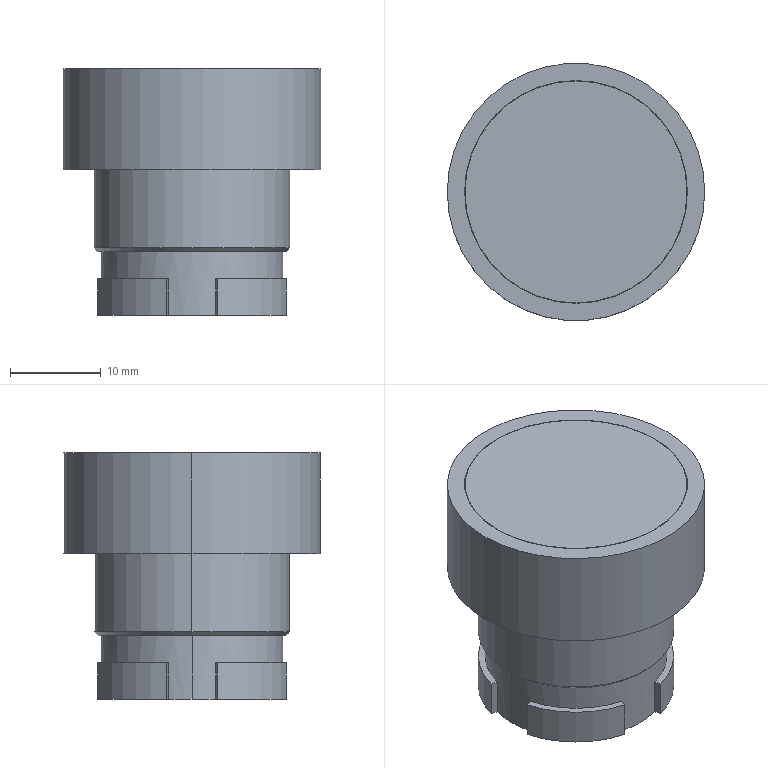Part | STEP file | 001. Yiweide green push-button switch EB6-BA31 | 1 solid | 40 faces | box 28.3 x 28.3 x 27.1 mm | volume 9249 mm3 | plane 20 | cylinder 18 | cone 2 | commonest cylinder face diameters 21.5 x6 18 x2 20 x2 24.4 x2 24.5 x2 26 x2
STEP:
#1=CARTESIAN_POINT('',(9.,0.,-4.));
#2=VERTEX_POINT('',#1);
#3=CARTESIAN_POINT('',(-9.,0.,-4.));
#4=VERTEX_POINT('',#3);
#5=CARTESIAN_POINT('',(0.,0.,-4.));
#6=DIRECTION('',(0.,0.,-1.));
#7=DIRECTION('',(-1.,0.,0.));
#8=AXIS2_PLACEMENT_3D('',#5,#6,#7);
#9=CIRCLE('',#8,9.);
#10=EDGE_CURVE('',#2,#4,#9,.T.);
#11=ORIENTED_EDGE('',*,*,#10,.F.);
#12=CARTESIAN_POINT('',(9.,0.,-16.));
#13=VERTEX_POINT('',#12);
#14=CARTESIAN_POINT('',(9.,0.,-4.));
#15=DIRECTION('',(0.,0.,-1.));
#16=VECTOR('',#15,1000.);
#17=LINE('',#14,#16);
#18=EDGE_CURVE('',#2,#13,#17,.T.);
#19=ORIENTED_EDGE('',*,*,#18,.T.);
#20=CARTESIAN_POINT('',(-9.,0.,-16.));
#21=VERTEX_POINT('',#20);
#22=CARTESIAN_POINT('',(0.,0.,-16.));
#23=DIRECTION('',(0.,0.,-1.));
#24=DIRECTION('',(-1.,0.,0.));
#25=AXIS2_PLACEMENT_3D('',#22,#23,#24);
#26=CIRCLE('',#25,9.);
#27=EDGE_CURVE('',#13,#21,#26,.T.);
#28=ORIENTED_EDGE('',*,*,#27,.T.);
#29=CARTESIAN_POINT('',(-9.,0.,-4.));
#30=DIRECTION('',(0.,0.,-1.));
#31=VECTOR('',#30,1000.);
#32=LINE('',#29,#31);
#33=EDGE_CURVE('',#4,#21,#32,.T.);
#34=ORIENTED_EDGE('',*,*,#33,.F.);
#35=EDGE_LOOP('',(#11,#19,#28,#34));
#36=FACE_OUTER_BOUND('',#35,.T.);
#37=CARTESIAN_POINT('',(0.,0.,-4.));
#38=DIRECTION('',(0.,0.,-1.));
#39=DIRECTION('',(-1.,0.,0.));
#40=AXIS2_PLACEMENT_3D('',#37,#38,#39);
#41=CYLINDRICAL_SURFACE('',#40,9.);
#42=ADVANCED_FACE('',(#36),#41,.F.);
#43=CARTESIAN_POINT('',(-10.35,0.,-9.));
#44=VERTEX_POINT('',#43);
#45=CARTESIAN_POINT('',(10.35,0.,-9.));
#46=VERTEX_POINT('',#45);
#47=CARTESIAN_POINT('',(0.,0.,-9.));
#48=DIRECTION('',(0.,0.,-1.));
#49=DIRECTION('',(-1.,0.,0.));
#50=AXIS2_PLACEMENT_3D('',#47,#48,#49);
#51=CIRCLE('',#50,10.35);
#52=EDGE_CURVE('',#44,#46,#51,.T.);
#53=ORIENTED_EDGE('',*,*,#52,.F.);
#54=CARTESIAN_POINT('',(-10.75,0.,-8.6));
#55=VERTEX_POINT('',#54);
#56=CARTESIAN_POINT('',(-10.35,0.,-9.));
#57=DIRECTION('',(-0.7071,0.,0.7071));
#58=VECTOR('',#57,1000.);
#59=LINE('',#56,#58);
#60=EDGE_CURVE('',#44,#55,#59,.T.);
#61=ORIENTED_EDGE('',*,*,#60,.T.);
#62=CARTESIAN_POINT('',(10.75,0.,-8.6));
#63=VERTEX_POINT('',#62);
#64=CARTESIAN_POINT('',(0.,0.,-8.6));
#65=DIRECTION('',(0.,0.,1.));
#66=DIRECTION('',(-1.,0.,0.));
#67=AXIS2_PLACEMENT_3D('',#64,#65,#66);
#68=CIRCLE('',#67,10.75);
#69=EDGE_CURVE('',#63,#55,#68,.T.);
#70=ORIENTED_EDGE('',*,*,#69,.F.);
#71=CARTESIAN_POINT('',(10.35,0.,-9.));
#72=DIRECTION('',(0.7071,0.,0.7071));
#73=VECTOR('',#72,1000.);
#74=LINE('',#71,#73);
#75=EDGE_CURVE('',#46,#63,#74,.T.);
#76=ORIENTED_EDGE('',*,*,#75,.F.);
#77=EDGE_LOOP('',(#53,#61,#70,#76));
#78=FACE_OUTER_BOUND('',#77,.T.);
#79=CARTESIAN_POINT('',(0.,0.,-9.));
#80=DIRECTION('',(0.,0.,1.));
#81=DIRECTION('',(1.,0.,0.));
#82=AXIS2_PLACEMENT_3D('',#79,#80,#81);
#83=CONICAL_SURFACE('',#82,10.35,0.7854);
#84=ADVANCED_FACE('',(#78),#83,.T.);
#85=CARTESIAN_POINT('',(-10.,0.,-9.));
#86=VERTEX_POINT('',#85);
#87=CARTESIAN_POINT('',(10.,0.,-9.));
#88=VERTEX_POINT('',#87);
#89=CARTESIAN_POINT('',(0.,0.,-9.));
#90=DIRECTION('',(0.,0.,-1.));
#91=DIRECTION('',(-1.,0.,0.));
#92=AXIS2_PLACEMENT_3D('',#89,#90,#91);
#93=CIRCLE('',#92,10.);
#94=EDGE_CURVE('',#86,#88,#93,.T.);
#95=ORIENTED_EDGE('',*,*,#94,.T.);
#96=CARTESIAN_POINT('',(10.,0.,-16.));
#97=VERTEX_POINT('',#96);
#98=CARTESIAN_POINT('',(10.,0.,-9.));
#99=DIRECTION('',(0.,0.,-1.));
#100=VECTOR('',#99,1000.);
#101=LINE('',#98,#100);
#102=EDGE_CURVE('',#88,#97,#101,.T.);
#103=ORIENTED_EDGE('',*,*,#102,.T.);
#104=CARTESIAN_POINT('',(9.659,2.588,-16.));
#105=VERTEX_POINT('',#104);
#106=CARTESIAN_POINT('',(0.,0.,-16.));
#107=DIRECTION('',(0.,0.,1.));
#108=DIRECTION('',(-1.,0.,0.));
#109=AXIS2_PLACEMENT_3D('',#106,#107,#108);
#110=CIRCLE('',#109,10.);
#111=EDGE_CURVE('',#97,#105,#110,.T.);
#112=ORIENTED_EDGE('',*,*,#111,.T.);
#113=CARTESIAN_POINT('',(9.659,2.588,-12.));
#114=VERTEX_POINT('',#113);
#115=CARTESIAN_POINT('',(9.659,2.588,11.101));
#116=DIRECTION('',(0.,0.,-1.));
#117=VECTOR('',#116,1000.);
#118=LINE('',#115,#117);
#119=EDGE_CURVE('',#114,#105,#118,.T.);
#120=ORIENTED_EDGE('',*,*,#119,.F.);
#121=CARTESIAN_POINT('',(2.588,9.659,-12.));
#122=VERTEX_POINT('',#121);
#123=CARTESIAN_POINT('',(0.,0.,-12.));
#124=DIRECTION('',(0.,0.,-1.));
#125=DIRECTION('',(-1.,0.,0.));
#126=AXIS2_PLACEMENT_3D('',#123,#124,#125);
#127=CIRCLE('',#126,10.);
#128=EDGE_CURVE('',#122,#114,#127,.T.);
#129=ORIENTED_EDGE('',*,*,#128,.F.);
#130=CARTESIAN_POINT('',(2.588,9.659,-16.));
#131=VERTEX_POINT('',#130);
#132=CARTESIAN_POINT('',(2.588,9.659,11.101));
#133=DIRECTION('',(0.,0.,-1.));
#134=VECTOR('',#133,1000.);
#135=LINE('',#132,#134);
#136=EDGE_CURVE('',#122,#131,#135,.T.);
#137=ORIENTED_EDGE('',*,*,#136,.T.);
#138=CARTESIAN_POINT('',(-2.588,9.659,-16.));
#139=VERTEX_POINT('',#138);
#140=CARTESIAN_POINT('',(0.,0.,-16.));
#141=DIRECTION('',(0.,0.,1.));
#142=DIRECTION('',(-1.,0.,0.));
#143=AXIS2_PLACEMENT_3D('',#140,#141,#142);
#144=CIRCLE('',#143,10.);
#145=EDGE_CURVE('',#131,#139,#144,.T.);
#146=ORIENTED_EDGE('',*,*,#145,.T.);
#147=CARTESIAN_POINT('',(-2.588,9.659,-12.));
#148=VERTEX_POINT('',#147);
#149=CARTESIAN_POINT('',(-2.588,9.659,11.101));
#150=DIRECTION('',(0.,0.,-1.));
#151=VECTOR('',#150,1000.);
#152=LINE('',#149,#151);
#153=EDGE_CURVE('',#148,#139,#152,.T.);
#154=ORIENTED_EDGE('',*,*,#153,.F.);
#155=CARTESIAN_POINT('',(-9.659,2.588,-12.));
#156=VERTEX_POINT('',#155);
#157=CARTESIAN_POINT('',(0.,0.,-12.));
#158=DIRECTION('',(0.,0.,-1.));
#159=DIRECTION('',(-1.,0.,0.));
#160=AXIS2_PLACEMENT_3D('',#157,#158,#159);
#161=CIRCLE('',#160,10.);
#162=EDGE_CURVE('',#156,#148,#161,.T.);
#163=ORIENTED_EDGE('',*,*,#162,.F.);
#164=CARTESIAN_POINT('',(-9.659,2.588,-16.));
#165=VERTEX_POINT('',#164);
#166=CARTESIAN_POINT('',(-9.659,2.588,11.101));
#167=DIRECTION('',(0.,0.,-1.));
#168=VECTOR('',#167,1000.);
#169=LINE('',#166,#168);
#170=EDGE_CURVE('',#156,#165,#169,.T.);
#171=ORIENTED_EDGE('',*,*,#170,.T.);
#172=CARTESIAN_POINT('',(-10.,0.,-16.));
#173=VERTEX_POINT('',#172);
#174=CARTESIAN_POINT('',(0.,0.,-16.));
#175=DIRECTION('',(0.,0.,1.));
#176=DIRECTION('',(-1.,0.,0.));
#177=AXIS2_PLACEMENT_3D('',#174,#175,#176);
#178=CIRCLE('',#177,10.);
#179=EDGE_CURVE('',#165,#173,#178,.T.);
#180=ORIENTED_EDGE('',*,*,#179,.T.);
#181=CARTESIAN_POINT('',(-10.,0.,-9.));
#182=DIRECTION('',(0.,0.,-1.));
#183=VECTOR('',#182,1000.);
#184=LINE('',#181,#183);
#185=EDGE_CURVE('',#86,#173,#184,.T.);
#186=ORIENTED_EDGE('',*,*,#185,.F.);
#187=EDGE_LOOP('',(#95,#103,#112,#120,#129,#137,#146,#154,#163,#171,#180,#186));
#188=FACE_OUTER_BOUND('',#187,.T.);
#189=CARTESIAN_POINT('',(0.,0.,-9.));
#190=DIRECTION('',(0.,0.,-1.));
#191=DIRECTION('',(-1.,0.,0.));
#192=AXIS2_PLACEMENT_3D('',#189,#190,#191);
#193=CYLINDRICAL_SURFACE('',#192,10.);
#194=ADVANCED_FACE('',(#188),#193,.T.);
#195=CARTESIAN_POINT('',(13.,0.,1.5));
#196=VERTEX_POINT('',#195);
#197=CARTESIAN_POINT('',(-13.,0.,1.5));
#198=VERTEX_POINT('',#197);
#199=CARTESIAN_POINT('',(0.,0.,1.5));
#200=DIRECTION('',(0.,0.,-1.));
#201=DIRECTION('',(-1.,0.,0.));
#202=AXIS2_PLACEMENT_3D('',#199,#200,#201);
#203=CIRCLE('',#202,13.);
#204=EDGE_CURVE('',#196,#198,#203,.T.);
#205=ORIENTED_EDGE('',*,*,#204,.F.);
#206=CARTESIAN_POINT('',(13.,0.,0.));
#207=VERTEX_POINT('',#206);
#208=CARTESIAN_POINT('',(13.,0.,1.5));
#209=DIRECTION('',(0.,0.,-1.));
#210=VECTOR('',#209,1000.);
#211=LINE('',#208,#210);
#212=EDGE_CURVE('',#196,#207,#211,.T.);
#213=ORIENTED_EDGE('',*,*,#212,.T.);
#214=CARTESIAN_POINT('',(-13.,0.,0.));
#215=VERTEX_POINT('',#214);
#216=CARTESIAN_POINT('',(0.,0.,0.));
#217=DIRECTION('',(0.,0.,-1.));
#218=DIRECTION('',(-1.,0.,0.));
#219=AXIS2_PLACEMENT_3D('',#216,#217,#218);
#220=CIRCLE('',#219,13.);
#221=EDGE_CURVE('',#207,#215,#220,.T.);
#222=ORIENTED_EDGE('',*,*,#221,.T.);
#223=CARTESIAN_POINT('',(-13.,0.,1.5));
#224=DIRECTION('',(0.,0.,-1.));
#225=VECTOR('',#224,1000.);
#226=LINE('',#223,#225);
#227=EDGE_CURVE('',#198,#215,#226,.T.);
#228=ORIENTED_EDGE('',*,*,#227,.F.);
#229=EDGE_LOOP('',(#205,#213,#222,#228));
#230=FACE_OUTER_BOUND('',#229,.T.);
#231=CARTESIAN_POINT('',(0.,0.,1.5));
#232=DIRECTION('',(0.,0.,-1.));
#233=DIRECTION('',(-1.,0.,0.));
#234=AXIS2_PLACEMENT_3D('',#231,#232,#233);
#235=CYLINDRICAL_SURFACE('',#234,13.);
#236=ADVANCED_FACE('',(#230),#235,.F.);
#237=CARTESIAN_POINT('',(12.2,0.,11.1));
#238=VERTEX_POINT('',#237);
#239=CARTESIAN_POINT('',(-12.2,0.,11.1));
#240=VERTEX_POINT('',#239);
#241=CARTESIAN_POINT('',(0.,0.,11.1));
#242=DIRECTION('',(0.,0.,1.));
#243=DIRECTION('',(1.,0.,0.));
#244=AXIS2_PLACEMENT_3D('',#241,#242,#243);
#245=CIRCLE('',#244,12.2);
#246=EDGE_CURVE('',#238,#240,#245,.T.);
#247=ORIENTED_EDGE('',*,*,#246,.F.);
#248=CARTESIAN_POINT('',(12.2,0.,6.1));
#249=VERTEX_POINT('',#248);
#250=CARTESIAN_POINT('',(12.2,0.,11.1));
#251=DIRECTION('',(0.,0.,-1.));
#252=VECTOR('',#251,1000.);
#253=LINE('',#250,#252);
#254=EDGE_CURVE('',#238,#249,#253,.T.);
#255=ORIENTED_EDGE('',*,*,#254,.T.);
#256=CARTESIAN_POINT('',(-12.2,0.,6.1));
#257=VERTEX_POINT('',#256);
#258=CARTESIAN_POINT('',(0.,0.,6.1));
#259=DIRECTION('',(0.,0.,1.));
#260=DIRECTION('',(1.,0.,0.));
#261=AXIS2_PLACEMENT_3D('',#258,#259,#260);
#262=CIRCLE('',#261,12.2);
#263=EDGE_CURVE('',#249,#257,#262,.T.);
#264=ORIENTED_EDGE('',*,*,#263,.T.);
#265=CARTESIAN_POINT('',(-12.2,0.,11.1));
#266=DIRECTION('',(0.,0.,-1.));
#267=VECTOR('',#266,1000.);
#268=LINE('',#265,#267);
#269=EDGE_CURVE('',#240,#257,#268,.T.);
#270=ORIENTED_EDGE('',*,*,#269,.F.);
#271=EDGE_LOOP('',(#247,#255,#264,#270));
#272=FACE_OUTER_BOUND('',#271,.T.);
#273=CARTESIAN_POINT('',(0.,0.,11.1));
#274=DIRECTION('',(0.,0.,-1.));
#275=DIRECTION('',(-1.,0.,0.));
#276=AXIS2_PLACEMENT_3D('',#273,#274,#275);
#277=CYLINDRICAL_SURFACE('',#276,12.2);
#278=ADVANCED_FACE('',(#272),#277,.T.);
#279=CARTESIAN_POINT('',(-12.25,0.,6.1));
#280=VERTEX_POINT('',#279);
#281=CARTESIAN_POINT('',(12.25,0.,6.1));
#282=VERTEX_POINT('',#281);
#283=CARTESIAN_POINT('',(0.,0.,6.1));
#284=DIRECTION('',(0.,0.,1.));
#285=DIRECTION('',(1.,0.,0.));
#286=AXIS2_PLACEMENT_3D('',#283,#284,#285);
#287=CIRCLE('',#286,12.25);
#288=EDGE_CURVE('',#280,#282,#287,.T.);
#289=ORIENTED_EDGE('',*,*,#288,.F.);
#290=CARTESIAN_POINT('',(-12.25,0.,11.1));
#291=VERTEX_POINT('',#290);
#292=CARTESIAN_POINT('',(-12.25,0.,6.1));
#293=DIRECTION('',(0.,0.,1.));
#294=VECTOR('',#293,1000.);
#295=LINE('',#292,#294);
#296=EDGE_CURVE('',#280,#291,#295,.T.);
#297=ORIENTED_EDGE('',*,*,#296,.T.);
#298=CARTESIAN_POINT('',(12.25,0.,11.1));
#299=VERTEX_POINT('',#298);
#300=CARTESIAN_POINT('',(0.,0.,11.1));
#301=DIRECTION('',(0.,0.,1.));
#302=DIRECTION('',(1.,0.,0.));
#303=AXIS2_PLACEMENT_3D('',#300,#301,#302);
#304=CIRCLE('',#303,12.25);
#305=EDGE_CURVE('',#291,#299,#304,.T.);
#306=ORIENTED_EDGE('',*,*,#305,.T.);
#307=CARTESIAN_POINT('',(12.25,0.,6.1));
#308=DIRECTION('',(0.,0.,1.));
#309=VECTOR('',#308,1000.);
#310=LINE('',#307,#309);
#311=EDGE_CURVE('',#282,#299,#310,.T.);
#312=ORIENTED_EDGE('',*,*,#311,.F.);
#313=EDGE_LOOP('',(#289,#297,#306,#312));
#314=FACE_OUTER_BOUND('',#313,.T.);
#315=CARTESIAN_POINT('',(0.,0.,6.1));
#316=DIRECTION('',(0.,0.,1.));
#317=DIRECTION('',(1.,0.,0.));
#318=AXIS2_PLACEMENT_3D('',#315,#316,#317);
#319=CYLINDRICAL_SURFACE('',#318,12.25);
#320=ADVANCED_FACE('',(#314),#319,.F.);
#321=CARTESIAN_POINT('',(14.15,0.,11.1));
#322=VERTEX_POINT('',#321);
#323=CARTESIAN_POINT('',(-14.15,0.,11.1));
#324=VERTEX_POINT('',#323);
#325=CARTESIAN_POINT('',(0.,0.,11.1));
#326=DIRECTION('',(0.,0.,1.));
#327=DIRECTION('',(1.,0.,0.));
#328=AXIS2_PLACEMENT_3D('',#325,#326,#327);
#329=CIRCLE('',#328,14.15);
#330=EDGE_CURVE('',#322,#324,#329,.T.);
#331=ORIENTED_EDGE('',*,*,#330,.F.);
#332=CARTESIAN_POINT('',(14.15,0.,0.));
#333=VERTEX_POINT('',#332);
#334=CARTESIAN_POINT('',(14.15,0.,11.1));
#335=DIRECTION('',(0.,0.,-1.));
#336=VECTOR('',#335,1000.);
#337=LINE('',#334,#336);
#338=EDGE_CURVE('',#322,#333,#337,.T.);
#339=ORIENTED_EDGE('',*,*,#338,.T.);
#340=CARTESIAN_POINT('',(-14.15,0.,0.));
#341=VERTEX_POINT('',#340);
#342=CARTESIAN_POINT('',(0.,0.,0.));
#343=DIRECTION('',(0.,0.,1.));
#344=DIRECTION('',(1.,0.,0.));
#345=AXIS2_PLACEMENT_3D('',#342,#343,#344);
#346=CIRCLE('',#345,14.15);
#347=EDGE_CURVE('',#333,#341,#346,.T.);
#348=ORIENTED_EDGE('',*,*,#347,.T.);
#349=CARTESIAN_POINT('',(-14.15,0.,11.1));
#350=DIRECTION('',(0.,0.,-1.));
#351=VECTOR('',#350,1000.);
#352=LINE('',#349,#351);
#353=EDGE_CURVE('',#324,#341,#352,.T.);
#354=ORIENTED_EDGE('',*,*,#353,.F.);
#355=EDGE_LOOP('',(#331,#339,#348,#354));
#356=FACE_OUTER_BOUND('',#355,.T.);
#357=CARTESIAN_POINT('',(0.,0.,11.1));
#358=DIRECTION('',(0.,0.,-1.));
#359=DIRECTION('',(-1.,0.,0.));
#360=AXIS2_PLACEMENT_3D('',#357,#358,#359);
#361=CYLINDRICAL_SURFACE('',#360,14.15);
#362=ADVANCED_FACE('',(#356),#361,.T.);
#363=ORIENTED_EDGE('',*,*,#69,.T.);
#364=CARTESIAN_POINT('',(-10.75,0.,1.5));
#365=VERTEX_POINT('',#364);
#366=CARTESIAN_POINT('',(-10.75,0.,-16.));
#367=DIRECTION('',(0.,0.,1.));
#368=VECTOR('',#367,1000.);
#369=LINE('',#366,#368);
#370=EDGE_CURVE('',#55,#365,#369,.T.);
#371=ORIENTED_EDGE('',*,*,#370,.T.);
#372=CARTESIAN_POINT('',(10.75,0.,1.5));
#373=VERTEX_POINT('',#372);
#374=CARTESIAN_POINT('',(0.,0.,1.5));
#375=DIRECTION('',(0.,0.,-1.));
#376=DIRECTION('',(-1.,0.,0.));
#377=AXIS2_PLACEMENT_3D('',#374,#375,#376);
#378=CIRCLE('',#377,10.75);
#379=EDGE_CURVE('',#365,#373,#378,.T.);
#380=ORIENTED_EDGE('',*,*,#379,.T.);
#381=CARTESIAN_POINT('',(10.75,0.,-16.));
#382=DIRECTION('',(0.,0.,1.));
#383=VECTOR('',#382,1000.);
#384=LINE('',#381,#383);
#385=EDGE_CURVE('',#63,#373,#384,.T.);
#386=ORIENTED_EDGE('',*,*,#385,.F.);
#387=EDGE_LOOP('',(#363,#371,#380,#386));
#388=FACE_OUTER_BOUND('',#387,.T.);
#389=CARTESIAN_POINT('',(0.,0.,-16.));
#390=DIRECTION('',(0.,0.,1.));
#391=DIRECTION('',(1.,0.,0.));
#392=AXIS2_PLACEMENT_3D('',#389,#390,#391);
#393=CYLINDRICAL_SURFACE('',#392,10.75);
#394=ADVANCED_FACE('',(#388),#393,.T.);
#395=CARTESIAN_POINT('',(-2.782,-10.384,-12.));
#396=VERTEX_POINT('',#395);
#397=CARTESIAN_POINT('',(-10.384,-2.782,-12.));
#398=VERTEX_POINT('',#397);
#399=CARTESIAN_POINT('',(0.,0.,-12.));
#400=DIRECTION('',(0.,0.,-1.));
#401=DIRECTION('',(-1.,0.,0.));
#402=AXIS2_PLACEMENT_3D('',#399,#400,#401);
#403=CIRCLE('',#402,10.75);
#404=EDGE_CURVE('',#396,#398,#403,.T.);
#405=ORIENTED_EDGE('',*,*,#404,.F.);
#406=CARTESIAN_POINT('',(-2.588,-9.659,-12.));
#407=VERTEX_POINT('',#406);
#408=CARTESIAN_POINT('',(-2.588,-9.659,-12.));
#409=DIRECTION('',(-0.2588,-0.9659,0.));
#410=VECTOR('',#409,1000.);
#411=LINE('',#408,#410);
#412=EDGE_CURVE('',#407,#396,#411,.T.);
#413=ORIENTED_EDGE('',*,*,#412,.F.);
#414=CARTESIAN_POINT('',(-9.659,-2.588,-12.));
#415=VERTEX_POINT('',#414);
#416=CARTESIAN_POINT('',(0.,0.,-12.));
#417=DIRECTION('',(0.,0.,-1.));
#418=DIRECTION('',(-1.,0.,0.));
#419=AXIS2_PLACEMENT_3D('',#416,#417,#418);
#420=CIRCLE('',#419,10.);
#421=EDGE_CURVE('',#407,#415,#420,.T.);
#422=ORIENTED_EDGE('',*,*,#421,.T.);
#423=CARTESIAN_POINT('',(-10.384,-2.782,-12.));
#424=DIRECTION('',(0.9659,0.2588,0.));
#425=VECTOR('',#424,1000.);
#426=LINE('',#423,#425);
#427=EDGE_CURVE('',#398,#415,#426,.T.);
#428=ORIENTED_EDGE('',*,*,#427,.F.);
#429=EDGE_LOOP('',(#405,#413,#422,#428));
#430=FACE_OUTER_BOUND('',#429,.T.);
#431=CARTESIAN_POINT('',(0.,0.,-12.));
#432=DIRECTION('',(0.,0.,-1.));
#433=DIRECTION('',(-1.,0.,0.));
#434=AXIS2_PLACEMENT_3D('',#431,#432,#433);
#435=PLANE('',#434);
#436=ADVANCED_FACE('',(#430),#435,.F.);
#437=CARTESIAN_POINT('',(-2.782,-10.384,-16.));
#438=VERTEX_POINT('',#437);
#439=CARTESIAN_POINT('',(-10.384,-2.782,-16.));
#440=VERTEX_POINT('',#439);
#441=CARTESIAN_POINT('',(0.,0.,-16.));
#442=DIRECTION('',(0.,0.,-1.));
#443=DIRECTION('',(-1.,0.,0.));
#444=AXIS2_PLACEMENT_3D('',#441,#442,#443);
#445=CIRCLE('',#444,10.75);
#446=EDGE_CURVE('',#438,#440,#445,.T.);
#447=ORIENTED_EDGE('',*,*,#446,.F.);
#448=CARTESIAN_POINT('',(-2.782,-10.384,11.101));
#449=DIRECTION('',(0.,0.,-1.));
#450=VECTOR('',#449,1000.);
#451=LINE('',#448,#450);
#452=EDGE_CURVE('',#396,#438,#451,.T.);
#453=ORIENTED_EDGE('',*,*,#452,.F.);
#454=ORIENTED_EDGE('',*,*,#404,.T.);
#455=CARTESIAN_POINT('',(-10.384,-2.782,11.101));
#456=DIRECTION('',(0.,0.,-1.));
#457=VECTOR('',#456,1000.);
#458=LINE('',#455,#457);
#459=EDGE_CURVE('',#398,#440,#458,.T.);
#460=ORIENTED_EDGE('',*,*,#459,.T.);
#461=EDGE_LOOP('',(#447,#453,#454,#460));
#462=FACE_OUTER_BOUND('',#461,.T.);
#463=CARTESIAN_POINT('',(0.,0.,-16.));
#464=DIRECTION('',(0.,0.,1.));
#465=DIRECTION('',(1.,0.,0.));
#466=AXIS2_PLACEMENT_3D('',#463,#464,#465);
#467=CYLINDRICAL_SURFACE('',#466,10.75);
#468=ADVANCED_FACE('',(#462),#467,.T.);
#469=ORIENTED_EDGE('',*,*,#128,.T.);
#470=CARTESIAN_POINT('',(10.384,2.782,-12.));
#471=VERTEX_POINT('',#470);
#472=CARTESIAN_POINT('',(9.659,2.588,-12.));
#473=DIRECTION('',(-0.9659,-0.2588,0.));
#474=VECTOR('',#473,1000.);
#475=LINE('',#472,#474);
#476=EDGE_CURVE('',#471,#114,#475,.T.);
#477=ORIENTED_EDGE('',*,*,#476,.F.);
#478=CARTESIAN_POINT('',(2.782,10.384,-12.));
#479=VERTEX_POINT('',#478);
#480=CARTESIAN_POINT('',(0.,0.,-12.));
#481=DIRECTION('',(0.,0.,-1.));
#482=DIRECTION('',(-1.,0.,0.));
#483=AXIS2_PLACEMENT_3D('',#480,#481,#482);
#484=CIRCLE('',#483,10.75);
#485=EDGE_CURVE('',#479,#471,#484,.T.);
#486=ORIENTED_EDGE('',*,*,#485,.F.);
#487=CARTESIAN_POINT('',(2.782,10.384,-12.));
#488=DIRECTION('',(0.2588,0.9659,0.));
#489=VECTOR('',#488,1000.);
#490=LINE('',#487,#489);
#491=EDGE_CURVE('',#122,#479,#490,.T.);
#492=ORIENTED_EDGE('',*,*,#491,.F.);
#493=EDGE_LOOP('',(#469,#477,#486,#492));
#494=FACE_OUTER_BOUND('',#493,.T.);
#495=CARTESIAN_POINT('',(0.,0.,-12.));
#496=DIRECTION('',(0.,0.,-1.));
#497=DIRECTION('',(-1.,0.,0.));
#498=AXIS2_PLACEMENT_3D('',#495,#496,#497);
#499=PLANE('',#498);
#500=ADVANCED_FACE('',(#494),#499,.F.);
#501=ORIENTED_EDGE('',*,*,#485,.T.);
#502=CARTESIAN_POINT('',(10.384,2.782,-16.));
#503=VERTEX_POINT('',#502);
#504=CARTESIAN_POINT('',(10.384,2.782,11.101));
#505=DIRECTION('',(0.,0.,-1.));
#506=VECTOR('',#505,1000.);
#507=LINE('',#504,#506);
#508=EDGE_CURVE('',#471,#503,#507,.T.);
#509=ORIENTED_EDGE('',*,*,#508,.T.);
#510=CARTESIAN_POINT('',(2.782,10.384,-16.));
#511=VERTEX_POINT('',#510);
#512=CARTESIAN_POINT('',(0.,0.,-16.));
#513=DIRECTION('',(0.,0.,-1.));
#514=DIRECTION('',(-1.,0.,0.));
#515=AXIS2_PLACEMENT_3D('',#512,#513,#514);
#516=CIRCLE('',#515,10.75);
#517=EDGE_CURVE('',#511,#503,#516,.T.);
#518=ORIENTED_EDGE('',*,*,#517,.F.);
#519=CARTESIAN_POINT('',(2.782,10.384,11.101));
#520=DIRECTION('',(0.,0.,-1.));
#521=VECTOR('',#520,1000.);
#522=LINE('',#519,#521);
#523=EDGE_CURVE('',#479,#511,#522,.T.);
#524=ORIENTED_EDGE('',*,*,#523,.F.);
#525=EDGE_LOOP('',(#501,#509,#518,#524));
#526=FACE_OUTER_BOUND('',#525,.T.);
#527=CARTESIAN_POINT('',(0.,0.,-16.));
#528=DIRECTION('',(0.,0.,1.));
#529=DIRECTION('',(1.,0.,0.));
#530=AXIS2_PLACEMENT_3D('',#527,#528,#529);
#531=CYLINDRICAL_SURFACE('',#530,10.75);
#532=ADVANCED_FACE('',(#526),#531,.T.);
#533=CARTESIAN_POINT('',(9.659,-2.588,-12.));
#534=VERTEX_POINT('',#533);
#535=CARTESIAN_POINT('',(2.588,-9.659,-12.));
#536=VERTEX_POINT('',#535);
#537=CARTESIAN_POINT('',(0.,0.,-12.));
#538=DIRECTION('',(0.,0.,-1.));
#539=DIRECTION('',(-1.,0.,0.));
#540=AXIS2_PLACEMENT_3D('',#537,#538,#539);
#541=CIRCLE('',#540,10.);
#542=EDGE_CURVE('',#534,#536,#541,.T.);
#543=ORIENTED_EDGE('',*,*,#542,.T.);
#544=CARTESIAN_POINT('',(2.782,-10.384,-12.));
#545=VERTEX_POINT('',#544);
#546=CARTESIAN_POINT('',(2.588,-9.659,-12.));
#547=DIRECTION('',(-0.2588,0.9659,0.));
#548=VECTOR('',#547,1000.);
#549=LINE('',#546,#548);
#550=EDGE_CURVE('',#545,#536,#549,.T.);
#551=ORIENTED_EDGE('',*,*,#550,.F.);
#552=CARTESIAN_POINT('',(10.384,-2.782,-12.));
#553=VERTEX_POINT('',#552);
#554=CARTESIAN_POINT('',(0.,0.,-12.));
#555=DIRECTION('',(0.,0.,-1.));
#556=DIRECTION('',(-1.,0.,0.));
#557=AXIS2_PLACEMENT_3D('',#554,#555,#556);
#558=CIRCLE('',#557,10.75);
#559=EDGE_CURVE('',#553,#545,#558,.T.);
#560=ORIENTED_EDGE('',*,*,#559,.F.);
#561=CARTESIAN_POINT('',(10.384,-2.782,-12.));
#562=DIRECTION('',(0.9659,-0.2588,0.));
#563=VECTOR('',#562,1000.);
#564=LINE('',#561,#563);
#565=EDGE_CURVE('',#534,#553,#564,.T.);
#566=ORIENTED_EDGE('',*,*,#565,.F.);
#567=EDGE_LOOP('',(#543,#551,#560,#566));
#568=FACE_OUTER_BOUND('',#567,.T.);
#569=CARTESIAN_POINT('',(0.,0.,-12.));
#570=DIRECTION('',(0.,0.,-1.));
#571=DIRECTION('',(-1.,0.,0.));
#572=AXIS2_PLACEMENT_3D('',#569,#570,#571);
#573=PLANE('',#572);
#574=ADVANCED_FACE('',(#568),#573,.F.);
#575=ORIENTED_EDGE('',*,*,#559,.T.);
#576=CARTESIAN_POINT('',(2.782,-10.384,-16.));
#577=VERTEX_POINT('',#576);
#578=CARTESIAN_POINT('',(2.782,-10.384,11.101));
#579=DIRECTION('',(0.,0.,-1.));
#580=VECTOR('',#579,1000.);
#581=LINE('',#578,#580);
#582=EDGE_CURVE('',#545,#577,#581,.T.);
#583=ORIENTED_EDGE('',*,*,#582,.T.);
#584=CARTESIAN_POINT('',(10.384,-2.782,-16.));
#585=VERTEX_POINT('',#584);
#586=CARTESIAN_POINT('',(0.,0.,-16.));
#587=DIRECTION('',(0.,0.,-1.));
#588=DIRECTION('',(-1.,0.,0.));
#589=AXIS2_PLACEMENT_3D('',#586,#587,#588);
#590=CIRCLE('',#589,10.75);
#591=EDGE_CURVE('',#585,#577,#590,.T.);
#592=ORIENTED_EDGE('',*,*,#591,.F.);
#593=CARTESIAN_POINT('',(10.384,-2.782,11.101));
#594=DIRECTION('',(0.,0.,-1.));
#595=VECTOR('',#594,1000.);
#596=LINE('',#593,#595);
#597=EDGE_CURVE('',#553,#585,#596,.T.);
#598=ORIENTED_EDGE('',*,*,#597,.F.);
#599=EDGE_LOOP('',(#575,#583,#592,#598));
#600=FACE_OUTER_BOUND('',#599,.T.);
#601=CARTESIAN_POINT('',(0.,0.,-16.));
#602=DIRECTION('',(0.,0.,1.));
#603=DIRECTION('',(1.,0.,0.));
#604=AXIS2_PLACEMENT_3D('',#601,#602,#603);
#605=CYLINDRICAL_SURFACE('',#604,10.75);
#606=ADVANCED_FACE('',(#600),#605,.T.);
#607=ORIENTED_EDGE('',*,*,#370,.F.);
#608=CARTESIAN_POINT('',(0.,0.,-8.6));
#609=DIRECTION('',(0.,0.,1.));
#610=DIRECTION('',(-1.,0.,0.));
#611=AXIS2_PLACEMENT_3D('',#608,#609,#610);
#612=CIRCLE('',#611,10.75);
#613=EDGE_CURVE('',#55,#63,#612,.T.);
#614=ORIENTED_EDGE('',*,*,#613,.T.);
#615=ORIENTED_EDGE('',*,*,#385,.T.);
#616=CARTESIAN_POINT('',(0.,0.,1.5));
#617=DIRECTION('',(0.,0.,-1.));
#618=DIRECTION('',(-1.,0.,0.));
#619=AXIS2_PLACEMENT_3D('',#616,#617,#618);
#620=CIRCLE('',#619,10.75);
#621=EDGE_CURVE('',#373,#365,#620,.T.);
#622=ORIENTED_EDGE('',*,*,#621,.T.);
#623=EDGE_LOOP('',(#607,#614,#615,#622));
#624=FACE_OUTER_BOUND('',#623,.T.);
#625=CARTESIAN_POINT('',(0.,0.,-16.));
#626=DIRECTION('',(0.,0.,1.));
#627=DIRECTION('',(1.,0.,0.));
#628=AXIS2_PLACEMENT_3D('',#625,#626,#627);
#629=CYLINDRICAL_SURFACE('',#628,10.75);
#630=ADVANCED_FACE('',(#624),#629,.T.);
#631=CARTESIAN_POINT('',(0.,0.,6.1));
#632=DIRECTION('',(0.,0.,1.));
#633=DIRECTION('',(1.,0.,0.));
#634=AXIS2_PLACEMENT_3D('',#631,#632,#633);
#635=CIRCLE('',#634,12.25);
#636=EDGE_CURVE('',#282,#280,#635,.T.);
#637=ORIENTED_EDGE('',*,*,#636,.T.);
#638=ORIENTED_EDGE('',*,*,#288,.T.);
#639=EDGE_LOOP('',(#637,#638));
#640=FACE_OUTER_BOUND('',#639,.T.);
#641=CARTESIAN_POINT('',(0.,0.,6.1));
#642=DIRECTION('',(0.,0.,1.));
#643=DIRECTION('',(1.,0.,0.));
#644=AXIS2_PLACEMENT_3D('',#641,#642,#643);
#645=CIRCLE('',#644,12.2);
#646=EDGE_CURVE('',#257,#249,#645,.T.);
#647=ORIENTED_EDGE('',*,*,#646,.F.);
#648=ORIENTED_EDGE('',*,*,#263,.F.);
#649=EDGE_LOOP('',(#647,#648));
#650=FACE_BOUND('',#649,.T.);
#651=CARTESIAN_POINT('',(0.,0.,6.1));
#652=DIRECTION('',(0.,0.,1.));
#653=DIRECTION('',(1.,0.,0.));
#654=AXIS2_PLACEMENT_3D('',#651,#652,#653);
#655=PLANE('',#654);
#656=ADVANCED_FACE('',(#640,#650),#655,.T.);
#657=CARTESIAN_POINT('',(0.,0.,0.));
#658=DIRECTION('',(0.,0.,-1.));
#659=DIRECTION('',(-1.,0.,0.));
#660=AXIS2_PLACEMENT_3D('',#657,#658,#659);
#661=CIRCLE('',#660,13.);
#662=EDGE_CURVE('',#215,#207,#661,.T.);
#663=ORIENTED_EDGE('',*,*,#662,.F.);
#664=ORIENTED_EDGE('',*,*,#221,.F.);
#665=EDGE_LOOP('',(#663,#664));
#666=FACE_BOUND('',#665,.T.);
#667=CARTESIAN_POINT('',(0.,0.,0.));
#668=DIRECTION('',(0.,0.,1.));
#669=DIRECTION('',(1.,0.,0.));
#670=AXIS2_PLACEMENT_3D('',#667,#668,#669);
#671=CIRCLE('',#670,14.15);
#672=EDGE_CURVE('',#341,#333,#671,.T.);
#673=ORIENTED_EDGE('',*,*,#672,.F.);
#674=ORIENTED_EDGE('',*,*,#347,.F.);
#675=EDGE_LOOP('',(#673,#674));
#676=FACE_OUTER_BOUND('',#675,.T.);
#677=CARTESIAN_POINT('',(0.,0.,0.));
#678=DIRECTION('',(0.,0.,1.));
#679=DIRECTION('',(1.,0.,0.));
#680=AXIS2_PLACEMENT_3D('',#677,#678,#679);
#681=PLANE('',#680);
#682=ADVANCED_FACE('',(#666,#676),#681,.F.);
#683=ORIENTED_EDGE('',*,*,#338,.F.);
#684=CARTESIAN_POINT('',(0.,0.,11.1));
#685=DIRECTION('',(0.,0.,1.));
#686=DIRECTION('',(1.,0.,0.));
#687=AXIS2_PLACEMENT_3D('',#684,#685,#686);
#688=CIRCLE('',#687,14.15);
#689=EDGE_CURVE('',#324,#322,#688,.T.);
#690=ORIENTED_EDGE('',*,*,#689,.F.);
#691=ORIENTED_EDGE('',*,*,#353,.T.);
#692=ORIENTED_EDGE('',*,*,#672,.T.);
#693=EDGE_LOOP('',(#683,#690,#691,#692));
#694=FACE_OUTER_BOUND('',#693,.T.);
#695=CARTESIAN_POINT('',(0.,0.,11.1));
#696=DIRECTION('',(0.,0.,-1.));
#697=DIRECTION('',(-1.,0.,0.));
#698=AXIS2_PLACEMENT_3D('',#695,#696,#697);
#699=CYLINDRICAL_SURFACE('',#698,14.15);
#700=ADVANCED_FACE('',(#694),#699,.T.);
#701=CARTESIAN_POINT('',(0.,0.,11.1));
#702=DIRECTION('',(0.,0.,1.));
#703=DIRECTION('',(1.,0.,0.));
#704=AXIS2_PLACEMENT_3D('',#701,#702,#703);
#705=CIRCLE('',#704,12.25);
#706=EDGE_CURVE('',#299,#291,#705,.T.);
#707=ORIENTED_EDGE('',*,*,#706,.F.);
#708=ORIENTED_EDGE('',*,*,#305,.F.);
#709=EDGE_LOOP('',(#707,#708));
#710=FACE_BOUND('',#709,.T.);
#711=ORIENTED_EDGE('',*,*,#689,.T.);
#712=ORIENTED_EDGE('',*,*,#330,.T.);
#713=EDGE_LOOP('',(#711,#712));
#714=FACE_OUTER_BOUND('',#713,.T.);
#715=CARTESIAN_POINT('',(0.,0.,11.1));
#716=DIRECTION('',(0.,0.,1.));
#717=DIRECTION('',(1.,0.,0.));
#718=AXIS2_PLACEMENT_3D('',#715,#716,#717);
#719=PLANE('',#718);
#720=ADVANCED_FACE('',(#710,#714),#719,.T.);
#721=ORIENTED_EDGE('',*,*,#296,.F.);
#722=ORIENTED_EDGE('',*,*,#636,.F.);
#723=ORIENTED_EDGE('',*,*,#311,.T.);
#724=ORIENTED_EDGE('',*,*,#706,.T.);
#725=EDGE_LOOP('',(#721,#722,#723,#724));
#726=FACE_OUTER_BOUND('',#725,.T.);
#727=CARTESIAN_POINT('',(0.,0.,6.1));
#728=DIRECTION('',(0.,0.,1.));
#729=DIRECTION('',(1.,0.,0.));
#730=AXIS2_PLACEMENT_3D('',#727,#728,#729);
#731=CYLINDRICAL_SURFACE('',#730,12.25);
#732=ADVANCED_FACE('',(#726),#731,.F.);
#733=ORIENTED_EDGE('',*,*,#254,.F.);
#734=CARTESIAN_POINT('',(0.,0.,11.1));
#735=DIRECTION('',(0.,0.,1.));
#736=DIRECTION('',(1.,0.,0.));
#737=AXIS2_PLACEMENT_3D('',#734,#735,#736);
#738=CIRCLE('',#737,12.2);
#739=EDGE_CURVE('',#240,#238,#738,.T.);
#740=ORIENTED_EDGE('',*,*,#739,.F.);
#741=ORIENTED_EDGE('',*,*,#269,.T.);
#742=ORIENTED_EDGE('',*,*,#646,.T.);
#743=EDGE_LOOP('',(#733,#740,#741,#742));
#744=FACE_OUTER_BOUND('',#743,.T.);
#745=CARTESIAN_POINT('',(0.,0.,11.1));
#746=DIRECTION('',(0.,0.,-1.));
#747=DIRECTION('',(-1.,0.,0.));
#748=AXIS2_PLACEMENT_3D('',#745,#746,#747);
#749=CYLINDRICAL_SURFACE('',#748,12.2);
#750=ADVANCED_FACE('',(#744),#749,.T.);
#751=ORIENTED_EDGE('',*,*,#739,.T.);
#752=ORIENTED_EDGE('',*,*,#246,.T.);
#753=EDGE_LOOP('',(#751,#752));
#754=FACE_OUTER_BOUND('',#753,.T.);
#755=CARTESIAN_POINT('',(0.,0.,11.1));
#756=DIRECTION('',(0.,0.,1.));
#757=DIRECTION('',(1.,0.,0.));
#758=AXIS2_PLACEMENT_3D('',#755,#756,#757);
#759=PLANE('',#758);
#760=ADVANCED_FACE('',(#754),#759,.T.);
#761=ORIENTED_EDGE('',*,*,#212,.F.);
#762=CARTESIAN_POINT('',(0.,0.,1.5));
#763=DIRECTION('',(0.,0.,-1.));
#764=DIRECTION('',(-1.,0.,0.));
#765=AXIS2_PLACEMENT_3D('',#762,#763,#764);
#766=CIRCLE('',#765,13.);
#767=EDGE_CURVE('',#198,#196,#766,.T.);
#768=ORIENTED_EDGE('',*,*,#767,.F.);
#769=ORIENTED_EDGE('',*,*,#227,.T.);
#770=ORIENTED_EDGE('',*,*,#662,.T.);
#771=EDGE_LOOP('',(#761,#768,#769,#770));
#772=FACE_OUTER_BOUND('',#771,.T.);
#773=CARTESIAN_POINT('',(0.,0.,1.5));
#774=DIRECTION('',(0.,0.,-1.));
#775=DIRECTION('',(-1.,0.,0.));
#776=AXIS2_PLACEMENT_3D('',#773,#774,#775);
#777=CYLINDRICAL_SURFACE('',#776,13.);
#778=ADVANCED_FACE('',(#772),#777,.F.);
#779=ORIENTED_EDGE('',*,*,#621,.F.);
#780=ORIENTED_EDGE('',*,*,#379,.F.);
#781=EDGE_LOOP('',(#779,#780));
#782=FACE_BOUND('',#781,.T.);
#783=ORIENTED_EDGE('',*,*,#767,.T.);
#784=ORIENTED_EDGE('',*,*,#204,.T.);
#785=EDGE_LOOP('',(#783,#784));
#786=FACE_OUTER_BOUND('',#785,.T.);
#787=CARTESIAN_POINT('',(0.,0.,1.5));
#788=DIRECTION('',(0.,0.,-1.));
#789=DIRECTION('',(-1.,0.,0.));
#790=AXIS2_PLACEMENT_3D('',#787,#788,#789);
#791=PLANE('',#790);
#792=ADVANCED_FACE('',(#782,#786),#791,.T.);
#793=CARTESIAN_POINT('',(0.,0.,-9.));
#794=DIRECTION('',(0.,0.,-1.));
#795=DIRECTION('',(-1.,0.,0.));
#796=AXIS2_PLACEMENT_3D('',#793,#794,#795);
#797=CIRCLE('',#796,10.35);
#798=EDGE_CURVE('',#46,#44,#797,.T.);
#799=ORIENTED_EDGE('',*,*,#798,.T.);
#800=ORIENTED_EDGE('',*,*,#52,.T.);
#801=EDGE_LOOP('',(#799,#800));
#802=FACE_OUTER_BOUND('',#801,.T.);
#803=ORIENTED_EDGE('',*,*,#94,.F.);
#804=CARTESIAN_POINT('',(0.,0.,-9.));
#805=DIRECTION('',(0.,0.,-1.));
#806=DIRECTION('',(-1.,0.,0.));
#807=AXIS2_PLACEMENT_3D('',#804,#805,#806);
#808=CIRCLE('',#807,10.);
#809=EDGE_CURVE('',#88,#86,#808,.T.);
#810=ORIENTED_EDGE('',*,*,#809,.F.);
#811=EDGE_LOOP('',(#803,#810));
#812=FACE_BOUND('',#811,.T.);
#813=CARTESIAN_POINT('',(0.,0.,-9.));
#814=DIRECTION('',(0.,0.,-1.));
#815=DIRECTION('',(-1.,0.,0.));
#816=AXIS2_PLACEMENT_3D('',#813,#814,#815);
#817=PLANE('',#816);
#818=ADVANCED_FACE('',(#802,#812),#817,.T.);
#819=CARTESIAN_POINT('',(-10.384,2.782,-12.));
#820=VERTEX_POINT('',#819);
#821=CARTESIAN_POINT('',(-2.782,10.384,-12.));
#822=VERTEX_POINT('',#821);
#823=CARTESIAN_POINT('',(0.,0.,-12.));
#824=DIRECTION('',(0.,0.,-1.));
#825=DIRECTION('',(-1.,0.,0.));
#826=AXIS2_PLACEMENT_3D('',#823,#824,#825);
#827=CIRCLE('',#826,10.75);
#828=EDGE_CURVE('',#820,#822,#827,.T.);
#829=ORIENTED_EDGE('',*,*,#828,.F.);
#830=CARTESIAN_POINT('',(-10.384,2.782,-12.));
#831=DIRECTION('',(-0.9659,0.2588,0.));
#832=VECTOR('',#831,1000.);
#833=LINE('',#830,#832);
#834=EDGE_CURVE('',#156,#820,#833,.T.);
#835=ORIENTED_EDGE('',*,*,#834,.F.);
#836=ORIENTED_EDGE('',*,*,#162,.T.);
#837=CARTESIAN_POINT('',(-2.782,10.384,-12.));
#838=DIRECTION('',(0.2588,-0.9659,0.));
#839=VECTOR('',#838,1000.);
#840=LINE('',#837,#839);
#841=EDGE_CURVE('',#822,#148,#840,.T.);
#842=ORIENTED_EDGE('',*,*,#841,.F.);
#843=EDGE_LOOP('',(#829,#835,#836,#842));
#844=FACE_OUTER_BOUND('',#843,.T.);
#845=CARTESIAN_POINT('',(0.,0.,-12.));
#846=DIRECTION('',(0.,0.,-1.));
#847=DIRECTION('',(-1.,0.,0.));
#848=AXIS2_PLACEMENT_3D('',#845,#846,#847);
#849=PLANE('',#848);
#850=ADVANCED_FACE('',(#844),#849,.F.);
#851=ORIENTED_EDGE('',*,*,#102,.F.);
#852=ORIENTED_EDGE('',*,*,#809,.T.);
#853=ORIENTED_EDGE('',*,*,#185,.T.);
#854=CARTESIAN_POINT('',(-9.659,-2.588,-16.));
#855=VERTEX_POINT('',#854);
#856=CARTESIAN_POINT('',(0.,0.,-16.));
#857=DIRECTION('',(0.,0.,1.));
#858=DIRECTION('',(-1.,0.,0.));
#859=AXIS2_PLACEMENT_3D('',#856,#857,#858);
#860=CIRCLE('',#859,10.);
#861=EDGE_CURVE('',#173,#855,#860,.T.);
#862=ORIENTED_EDGE('',*,*,#861,.T.);
#863=CARTESIAN_POINT('',(-9.659,-2.588,11.101));
#864=DIRECTION('',(0.,0.,-1.));
#865=VECTOR('',#864,1000.);
#866=LINE('',#863,#865);
#867=EDGE_CURVE('',#415,#855,#866,.T.);
#868=ORIENTED_EDGE('',*,*,#867,.F.);
#869=ORIENTED_EDGE('',*,*,#421,.F.);
#870=CARTESIAN_POINT('',(-2.588,-9.659,-16.));
#871=VERTEX_POINT('',#870);
#872=CARTESIAN_POINT('',(-2.588,-9.659,11.101));
#873=DIRECTION('',(0.,0.,-1.));
#874=VECTOR('',#873,1000.);
#875=LINE('',#872,#874);
#876=EDGE_CURVE('',#407,#871,#875,.T.);
#877=ORIENTED_EDGE('',*,*,#876,.T.);
#878=CARTESIAN_POINT('',(2.588,-9.659,-16.));
#879=VERTEX_POINT('',#878);
#880=CARTESIAN_POINT('',(0.,0.,-16.));
#881=DIRECTION('',(0.,0.,1.));
#882=DIRECTION('',(-1.,0.,0.));
#883=AXIS2_PLACEMENT_3D('',#880,#881,#882);
#884=CIRCLE('',#883,10.);
#885=EDGE_CURVE('',#871,#879,#884,.T.);
#886=ORIENTED_EDGE('',*,*,#885,.T.);
#887=CARTESIAN_POINT('',(2.588,-9.659,11.101));
#888=DIRECTION('',(0.,0.,-1.));
#889=VECTOR('',#888,1000.);
#890=LINE('',#887,#889);
#891=EDGE_CURVE('',#536,#879,#890,.T.);
#892=ORIENTED_EDGE('',*,*,#891,.F.);
#893=ORIENTED_EDGE('',*,*,#542,.F.);
#894=CARTESIAN_POINT('',(9.659,-2.588,-16.));
#895=VERTEX_POINT('',#894);
#896=CARTESIAN_POINT('',(9.659,-2.588,11.101));
#897=DIRECTION('',(0.,0.,-1.));
#898=VECTOR('',#897,1000.);
#899=LINE('',#896,#898);
#900=EDGE_CURVE('',#534,#895,#899,.T.);
#901=ORIENTED_EDGE('',*,*,#900,.T.);
#902=CARTESIAN_POINT('',(0.,0.,-16.));
#903=DIRECTION('',(0.,0.,1.));
#904=DIRECTION('',(-1.,0.,0.));
#905=AXIS2_PLACEMENT_3D('',#902,#903,#904);
#906=CIRCLE('',#905,10.);
#907=EDGE_CURVE('',#895,#97,#906,.T.);
#908=ORIENTED_EDGE('',*,*,#907,.T.);
#909=EDGE_LOOP('',(#851,#852,#853,#862,#868,#869,#877,#886,#892,#893,#901,#908));
#910=FACE_OUTER_BOUND('',#909,.T.);
#911=CARTESIAN_POINT('',(0.,0.,-9.));
#912=DIRECTION('',(0.,0.,-1.));
#913=DIRECTION('',(-1.,0.,0.));
#914=AXIS2_PLACEMENT_3D('',#911,#912,#913);
#915=CYLINDRICAL_SURFACE('',#914,10.);
#916=ADVANCED_FACE('',(#910),#915,.T.);
#917=CARTESIAN_POINT('',(0.,0.,-16.));
#918=DIRECTION('',(0.,0.,-1.));
#919=DIRECTION('',(-1.,0.,0.));
#920=AXIS2_PLACEMENT_3D('',#917,#918,#919);
#921=CIRCLE('',#920,9.);
#922=EDGE_CURVE('',#21,#13,#921,.T.);
#923=ORIENTED_EDGE('',*,*,#922,.F.);
#924=ORIENTED_EDGE('',*,*,#27,.F.);
#925=EDGE_LOOP('',(#923,#924));
#926=FACE_BOUND('',#925,.T.);
#927=CARTESIAN_POINT('',(-2.588,-9.659,-16.));
#928=DIRECTION('',(0.2588,0.9659,0.));
#929=VECTOR('',#928,1000.);
#930=LINE('',#927,#929);
#931=EDGE_CURVE('',#438,#871,#930,.T.);
#932=ORIENTED_EDGE('',*,*,#931,.F.);
#933=ORIENTED_EDGE('',*,*,#446,.T.);
#934=CARTESIAN_POINT('',(-10.384,-2.782,-16.));
#935=DIRECTION('',(-0.9659,-0.2588,0.));
#936=VECTOR('',#935,1000.);
#937=LINE('',#934,#936);
#938=EDGE_CURVE('',#855,#440,#937,.T.);
#939=ORIENTED_EDGE('',*,*,#938,.F.);
#940=ORIENTED_EDGE('',*,*,#861,.F.);
#941=ORIENTED_EDGE('',*,*,#179,.F.);
#942=CARTESIAN_POINT('',(-10.384,2.782,-16.));
#943=VERTEX_POINT('',#942);
#944=CARTESIAN_POINT('',(-10.384,2.782,-16.));
#945=DIRECTION('',(0.9659,-0.2588,0.));
#946=VECTOR('',#945,1000.);
#947=LINE('',#944,#946);
#948=EDGE_CURVE('',#943,#165,#947,.T.);
#949=ORIENTED_EDGE('',*,*,#948,.F.);
#950=CARTESIAN_POINT('',(-2.782,10.384,-16.));
#951=VERTEX_POINT('',#950);
#952=CARTESIAN_POINT('',(0.,0.,-16.));
#953=DIRECTION('',(0.,0.,-1.));
#954=DIRECTION('',(-1.,0.,0.));
#955=AXIS2_PLACEMENT_3D('',#952,#953,#954);
#956=CIRCLE('',#955,10.75);
#957=EDGE_CURVE('',#943,#951,#956,.T.);
#958=ORIENTED_EDGE('',*,*,#957,.T.);
#959=CARTESIAN_POINT('',(-2.782,10.384,-16.));
#960=DIRECTION('',(-0.2588,0.9659,0.));
#961=VECTOR('',#960,1000.);
#962=LINE('',#959,#961);
#963=EDGE_CURVE('',#139,#951,#962,.T.);
#964=ORIENTED_EDGE('',*,*,#963,.F.);
#965=ORIENTED_EDGE('',*,*,#145,.F.);
#966=CARTESIAN_POINT('',(2.782,10.384,-16.));
#967=DIRECTION('',(-0.2588,-0.9659,0.));
#968=VECTOR('',#967,1000.);
#969=LINE('',#966,#968);
#970=EDGE_CURVE('',#511,#131,#969,.T.);
#971=ORIENTED_EDGE('',*,*,#970,.F.);
#972=ORIENTED_EDGE('',*,*,#517,.T.);
#973=CARTESIAN_POINT('',(9.659,2.588,-16.));
#974=DIRECTION('',(0.9659,0.2588,0.));
#975=VECTOR('',#974,1000.);
#976=LINE('',#973,#975);
#977=EDGE_CURVE('',#105,#503,#976,.T.);
#978=ORIENTED_EDGE('',*,*,#977,.F.);
#979=ORIENTED_EDGE('',*,*,#111,.F.);
#980=ORIENTED_EDGE('',*,*,#907,.F.);
#981=CARTESIAN_POINT('',(10.384,-2.782,-16.));
#982=DIRECTION('',(-0.9659,0.2588,0.));
#983=VECTOR('',#982,1000.);
#984=LINE('',#981,#983);
#985=EDGE_CURVE('',#585,#895,#984,.T.);
#986=ORIENTED_EDGE('',*,*,#985,.F.);
#987=ORIENTED_EDGE('',*,*,#591,.T.);
#988=CARTESIAN_POINT('',(2.588,-9.659,-16.));
#989=DIRECTION('',(0.2588,-0.9659,0.));
#990=VECTOR('',#989,1000.);
#991=LINE('',#988,#990);
#992=EDGE_CURVE('',#879,#577,#991,.T.);
#993=ORIENTED_EDGE('',*,*,#992,.F.);
#994=ORIENTED_EDGE('',*,*,#885,.F.);
#995=EDGE_LOOP('',(#932,#933,#939,#940,#941,#949,#958,#964,#965,#971,#972,#978,#979,#980,#986,#987,#993,#994));
#996=FACE_OUTER_BOUND('',#995,.T.);
#997=CARTESIAN_POINT('',(0.,0.,-16.));
#998=DIRECTION('',(0.,0.,-1.));
#999=DIRECTION('',(-1.,0.,0.));
#1000=AXIS2_PLACEMENT_3D('',#997,#998,#999);
#1001=PLANE('',#1000);
#1002=ADVANCED_FACE('',(#926,#996),#1001,.T.);
#1003=ORIENTED_EDGE('',*,*,#957,.F.);
#1004=CARTESIAN_POINT('',(-10.384,2.782,11.101));
#1005=DIRECTION('',(0.,0.,-1.));
#1006=VECTOR('',#1005,1000.);
#1007=LINE('',#1004,#1006);
#1008=EDGE_CURVE('',#820,#943,#1007,.T.);
#1009=ORIENTED_EDGE('',*,*,#1008,.F.);
#1010=ORIENTED_EDGE('',*,*,#828,.T.);
#1011=CARTESIAN_POINT('',(-2.782,10.384,11.101));
#1012=DIRECTION('',(0.,0.,-1.));
#1013=VECTOR('',#1012,1000.);
#1014=LINE('',#1011,#1013);
#1015=EDGE_CURVE('',#822,#951,#1014,.T.);
#1016=ORIENTED_EDGE('',*,*,#1015,.T.);
#1017=EDGE_LOOP('',(#1003,#1009,#1010,#1016));
#1018=FACE_OUTER_BOUND('',#1017,.T.);
#1019=CARTESIAN_POINT('',(0.,0.,-16.));
#1020=DIRECTION('',(0.,0.,1.));
#1021=DIRECTION('',(1.,0.,0.));
#1022=AXIS2_PLACEMENT_3D('',#1019,#1020,#1021);
#1023=CYLINDRICAL_SURFACE('',#1022,10.75);
#1024=ADVANCED_FACE('',(#1018),#1023,.T.);
#1025=ORIENTED_EDGE('',*,*,#60,.F.);
#1026=ORIENTED_EDGE('',*,*,#798,.F.);
#1027=ORIENTED_EDGE('',*,*,#75,.T.);
#1028=ORIENTED_EDGE('',*,*,#613,.F.);
#1029=EDGE_LOOP('',(#1025,#1026,#1027,#1028));
#1030=FACE_OUTER_BOUND('',#1029,.T.);
#1031=CARTESIAN_POINT('',(0.,0.,-9.));
#1032=DIRECTION('',(0.,0.,1.));
#1033=DIRECTION('',(1.,0.,0.));
#1034=AXIS2_PLACEMENT_3D('',#1031,#1032,#1033);
#1035=CONICAL_SURFACE('',#1034,10.35,0.7854);
#1036=ADVANCED_FACE('',(#1030),#1035,.T.);
#1037=ORIENTED_EDGE('',*,*,#841,.T.);
#1038=ORIENTED_EDGE('',*,*,#153,.T.);
#1039=ORIENTED_EDGE('',*,*,#963,.T.);
#1040=ORIENTED_EDGE('',*,*,#1015,.F.);
#1041=EDGE_LOOP('',(#1037,#1038,#1039,#1040));
#1042=FACE_OUTER_BOUND('',#1041,.T.);
#1043=CARTESIAN_POINT('',(-2.782,10.384,11.101));
#1044=DIRECTION('',(-0.9659,-0.2588,0.));
#1045=DIRECTION('',(0.2588,-0.9659,0.));
#1046=AXIS2_PLACEMENT_3D('',#1043,#1044,#1045);
#1047=PLANE('',#1046);
#1048=ADVANCED_FACE('',(#1042),#1047,.F.);
#1049=ORIENTED_EDGE('',*,*,#491,.T.);
#1050=ORIENTED_EDGE('',*,*,#523,.T.);
#1051=ORIENTED_EDGE('',*,*,#970,.T.);
#1052=ORIENTED_EDGE('',*,*,#136,.F.);
#1053=EDGE_LOOP('',(#1049,#1050,#1051,#1052));
#1054=FACE_OUTER_BOUND('',#1053,.T.);
#1055=CARTESIAN_POINT('',(2.782,10.384,11.101));
#1056=DIRECTION('',(0.9659,-0.2588,0.));
#1057=DIRECTION('',(0.2588,0.9659,0.));
#1058=AXIS2_PLACEMENT_3D('',#1055,#1056,#1057);
#1059=PLANE('',#1058);
#1060=ADVANCED_FACE('',(#1054),#1059,.F.);
#1061=ORIENTED_EDGE('',*,*,#427,.T.);
#1062=ORIENTED_EDGE('',*,*,#867,.T.);
#1063=ORIENTED_EDGE('',*,*,#938,.T.);
#1064=ORIENTED_EDGE('',*,*,#459,.F.);
#1065=EDGE_LOOP('',(#1061,#1062,#1063,#1064));
#1066=FACE_OUTER_BOUND('',#1065,.T.);
#1067=CARTESIAN_POINT('',(-10.384,-2.782,11.101));
#1068=DIRECTION('',(0.2588,-0.9659,0.));
#1069=DIRECTION('',(0.9659,0.2588,0.));
#1070=AXIS2_PLACEMENT_3D('',#1067,#1068,#1069);
#1071=PLANE('',#1070);
#1072=ADVANCED_FACE('',(#1066),#1071,.F.);
#1073=ORIENTED_EDGE('',*,*,#834,.T.);
#1074=ORIENTED_EDGE('',*,*,#1008,.T.);
#1075=ORIENTED_EDGE('',*,*,#948,.T.);
#1076=ORIENTED_EDGE('',*,*,#170,.F.);
#1077=EDGE_LOOP('',(#1073,#1074,#1075,#1076));
#1078=FACE_OUTER_BOUND('',#1077,.T.);
#1079=CARTESIAN_POINT('',(-10.384,2.782,11.101));
#1080=DIRECTION('',(0.2588,0.9659,0.));
#1081=DIRECTION('',(-0.9659,0.2588,0.));
#1082=AXIS2_PLACEMENT_3D('',#1079,#1080,#1081);
#1083=PLANE('',#1082);
#1084=ADVANCED_FACE('',(#1078),#1083,.F.);
#1085=ORIENTED_EDGE('',*,*,#476,.T.);
#1086=ORIENTED_EDGE('',*,*,#119,.T.);
#1087=ORIENTED_EDGE('',*,*,#977,.T.);
#1088=ORIENTED_EDGE('',*,*,#508,.F.);
#1089=EDGE_LOOP('',(#1085,#1086,#1087,#1088));
#1090=FACE_OUTER_BOUND('',#1089,.T.);
#1091=CARTESIAN_POINT('',(9.659,2.588,11.101));
#1092=DIRECTION('',(-0.2588,0.9659,0.));
#1093=DIRECTION('',(-0.9659,-0.2588,0.));
#1094=AXIS2_PLACEMENT_3D('',#1091,#1092,#1093);
#1095=PLANE('',#1094);
#1096=ADVANCED_FACE('',(#1090),#1095,.F.);
#1097=ORIENTED_EDGE('',*,*,#565,.T.);
#1098=ORIENTED_EDGE('',*,*,#597,.T.);
#1099=ORIENTED_EDGE('',*,*,#985,.T.);
#1100=ORIENTED_EDGE('',*,*,#900,.F.);
#1101=EDGE_LOOP('',(#1097,#1098,#1099,#1100));
#1102=FACE_OUTER_BOUND('',#1101,.T.);
#1103=CARTESIAN_POINT('',(10.384,-2.782,11.101));
#1104=DIRECTION('',(-0.2588,-0.9659,0.));
#1105=DIRECTION('',(0.9659,-0.2588,0.));
#1106=AXIS2_PLACEMENT_3D('',#1103,#1104,#1105);
#1107=PLANE('',#1106);
#1108=ADVANCED_FACE('',(#1102),#1107,.F.);
#1109=ORIENTED_EDGE('',*,*,#412,.T.);
#1110=ORIENTED_EDGE('',*,*,#452,.T.);
#1111=ORIENTED_EDGE('',*,*,#931,.T.);
#1112=ORIENTED_EDGE('',*,*,#876,.F.);
#1113=EDGE_LOOP('',(#1109,#1110,#1111,#1112));
#1114=FACE_OUTER_BOUND('',#1113,.T.);
#1115=CARTESIAN_POINT('',(-2.588,-9.659,11.101));
#1116=DIRECTION('',(-0.9659,0.2588,0.));
#1117=DIRECTION('',(-0.2588,-0.9659,0.));
#1118=AXIS2_PLACEMENT_3D('',#1115,#1116,#1117);
#1119=PLANE('',#1118);
#1120=ADVANCED_FACE('',(#1114),#1119,.F.);
#1121=ORIENTED_EDGE('',*,*,#550,.T.);
#1122=ORIENTED_EDGE('',*,*,#891,.T.);
#1123=ORIENTED_EDGE('',*,*,#992,.T.);
#1124=ORIENTED_EDGE('',*,*,#582,.F.);
#1125=EDGE_LOOP('',(#1121,#1122,#1123,#1124));
#1126=FACE_OUTER_BOUND('',#1125,.T.);
#1127=CARTESIAN_POINT('',(2.588,-9.659,11.101));
#1128=DIRECTION('',(0.9659,0.2588,0.));
#1129=DIRECTION('',(-0.2588,0.9659,0.));
#1130=AXIS2_PLACEMENT_3D('',#1127,#1128,#1129);
#1131=PLANE('',#1130);
#1132=ADVANCED_FACE('',(#1126),#1131,.F.);
#1133=ORIENTED_EDGE('',*,*,#18,.F.);
#1134=CARTESIAN_POINT('',(0.,0.,-4.));
#1135=DIRECTION('',(0.,0.,-1.));
#1136=DIRECTION('',(-1.,0.,0.));
#1137=AXIS2_PLACEMENT_3D('',#1134,#1135,#1136);
#1138=CIRCLE('',#1137,9.);
#1139=EDGE_CURVE('',#4,#2,#1138,.T.);
#1140=ORIENTED_EDGE('',*,*,#1139,.F.);
#1141=ORIENTED_EDGE('',*,*,#33,.T.);
#1142=ORIENTED_EDGE('',*,*,#922,.T.);
#1143=EDGE_LOOP('',(#1133,#1140,#1141,#1142));
#1144=FACE_OUTER_BOUND('',#1143,.T.);
#1145=CARTESIAN_POINT('',(0.,0.,-4.));
#1146=DIRECTION('',(0.,0.,-1.));
#1147=DIRECTION('',(-1.,0.,0.));
#1148=AXIS2_PLACEMENT_3D('',#1145,#1146,#1147);
#1149=CYLINDRICAL_SURFACE('',#1148,9.);
#1150=ADVANCED_FACE('',(#1144),#1149,.F.);
#1151=ORIENTED_EDGE('',*,*,#1139,.T.);
#1152=ORIENTED_EDGE('',*,*,#10,.T.);
#1153=EDGE_LOOP('',(#1151,#1152));
#1154=FACE_OUTER_BOUND('',#1153,.T.);
#1155=CARTESIAN_POINT('',(0.,0.,-4.));
#1156=DIRECTION('',(0.,0.,-1.));
#1157=DIRECTION('',(-1.,0.,0.));
#1158=AXIS2_PLACEMENT_3D('',#1155,#1156,#1157);
#1159=PLANE('',#1158);
#1160=ADVANCED_FACE('',(#1154),#1159,.T.);
#1161=CLOSED_SHELL('',(#42,#84,#194,#236,#278,#320,#362,#394,#436,#468,#500,#532,#574,#606,#630,#656,#682,#700,#720,#732,#750,#760,#778,#792,#818,#850,#916,#1002,#1024,#1036,#1048,#1060,#1072,#1084,#1096,#1108,#1120,#1132,#1150,#1160));
#1162=MANIFOLD_SOLID_BREP('',#1161);
#1163=CARTESIAN_POINT('',(0.,0.,0.));
#1164=DIRECTION('',(0.,0.,1.));
#1165=DIRECTION('',(1.,0.,0.));
#1166=AXIS2_PLACEMENT_3D('',#1163,#1164,#1165);
#1167=(LENGTH_UNIT()NAMED_UNIT(*)SI_UNIT(.MILLI.,.METRE.));
#1168=UNCERTAINTY_MEASURE_WITH_UNIT(LENGTH_MEASURE(0.00001),#1167,'','');
#1169=(NAMED_UNIT(*)PLANE_ANGLE_UNIT()SI_UNIT($,.RADIAN.));
#1170=(NAMED_UNIT(*)SI_UNIT($,.STERADIAN.)SOLID_ANGLE_UNIT());
#1171=(GEOMETRIC_REPRESENTATION_CONTEXT(3)GLOBAL_UNCERTAINTY_ASSIGNED_CONTEXT((#1168))GLOBAL_UNIT_ASSIGNED_CONTEXT((#1167,#1169,#1170))REPRESENTATION_CONTEXT('',''));
#1172=ADVANCED_BREP_SHAPE_REPRESENTATION('',(#1162,#1166),#1171);